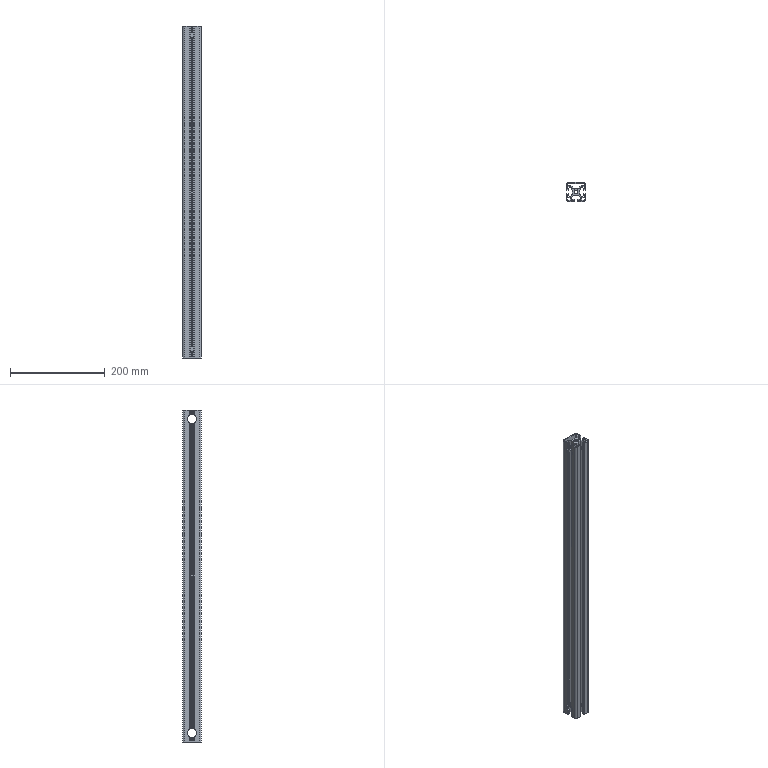Part | SolidWorks | features BaseBody 1, HoleWzd 1, MoveFace 1 | 1 solid | 242 faces | box 40 x 40 x 700 mm | volume 406067 mm3 | plane 187 | cylinder 55 | commonest cylinder face diameters 6.8 x15 2 x14 19 x12 1 x6 5 x4 9 x4